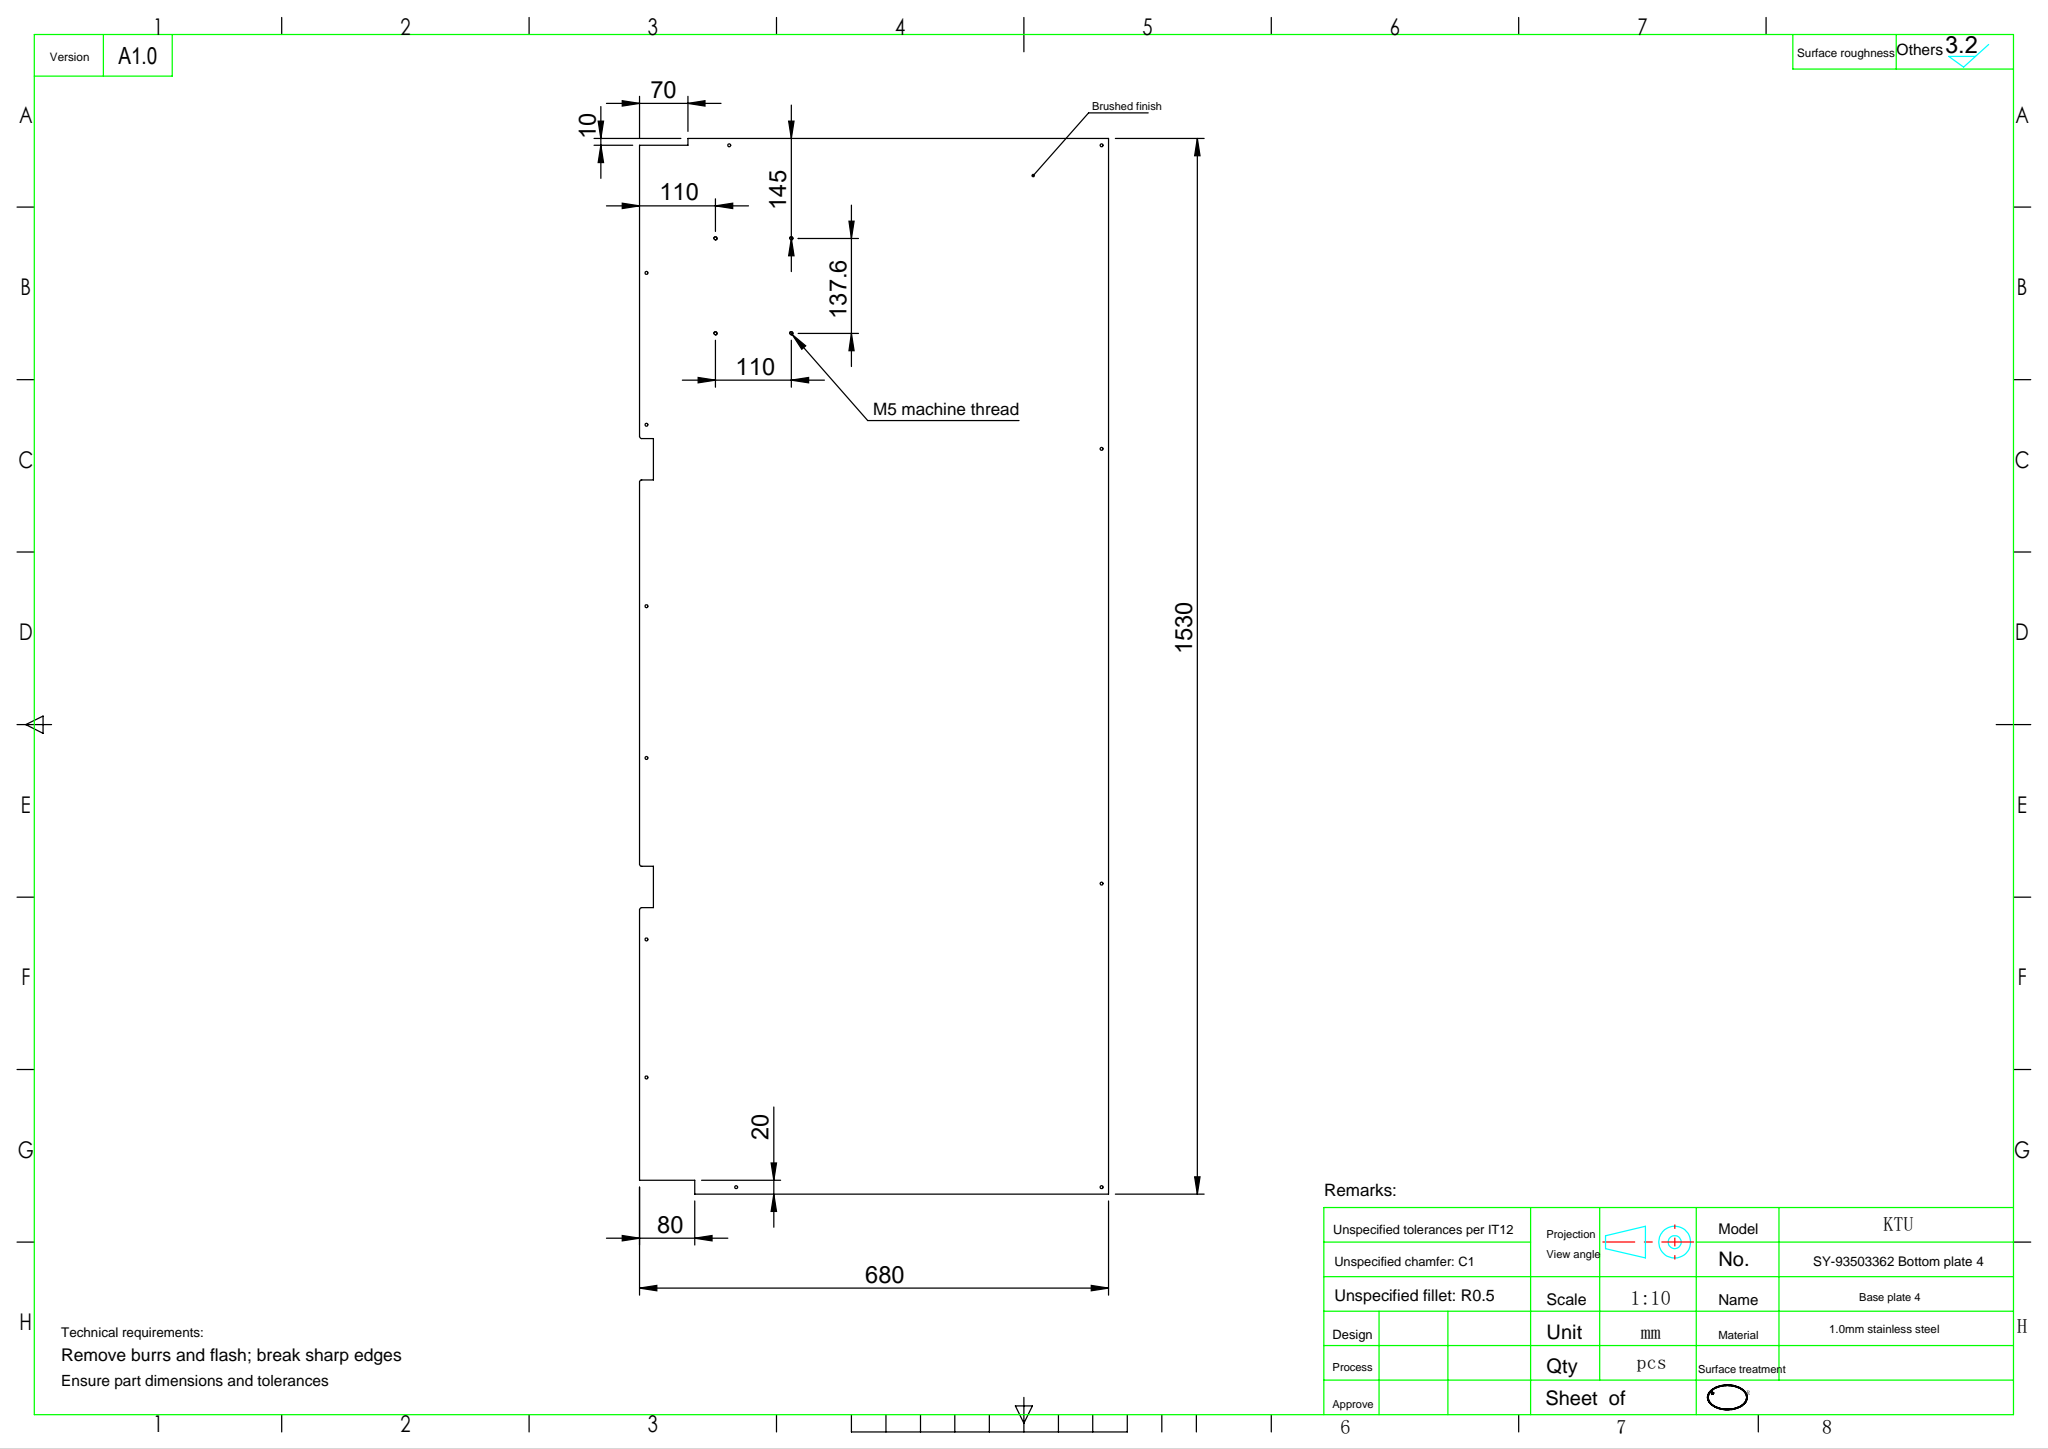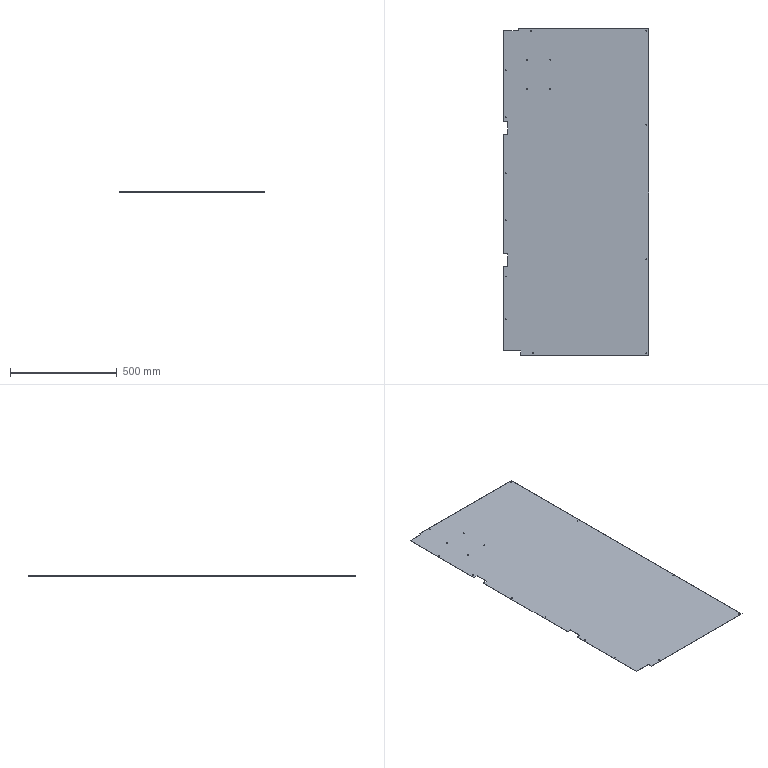Part | SolidWorks | features Cut 3, Fillet 1, FlatPattern 1, ICE 1, SMBaseFlange 1, SheetMetal 1 | 1 solid | 54 faces | box 680 x 1530 x 1 mm | volume 1035471 mm3 | cylinder 36 | plane 18 | commonest cylinder face diameters 4.2 x32 6 x4